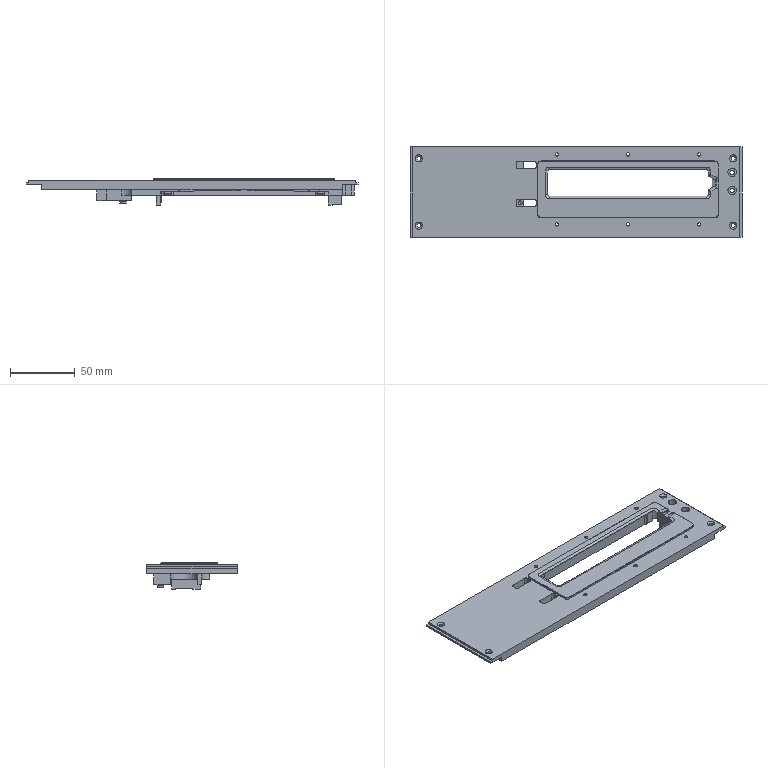Part | 1 solid | 266 faces | box 256.6 x 70.3 x 20.422 mm | volume 112249 mm3 | plane 139 | cylinder 93 | cone 24 | spline 10 | commonest cylinder face diameters 3.2 x25 2 x16 2.6 x14 6 x12 4 x8 3.4 x4